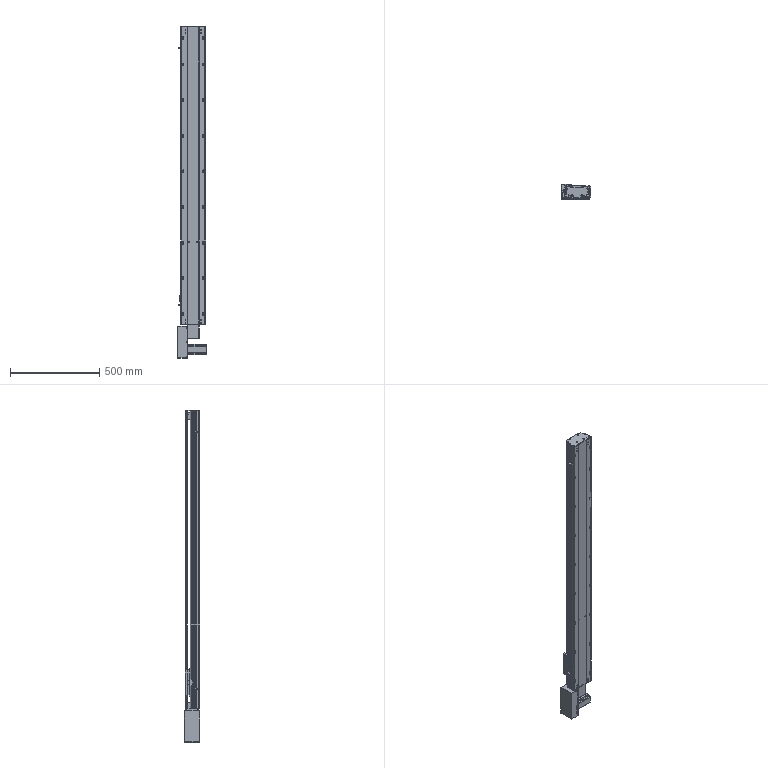Part | SolidWorks | 45 solids | 3321 faces | volume 6114333 mm3 | cylinder 2141 | plane 738 | cone 322 | torus 120 | commonest cylinder face diameters 1.1 x287 0.5 x280 6.55 x262 5 x133 4.5 x84 6.6 x72